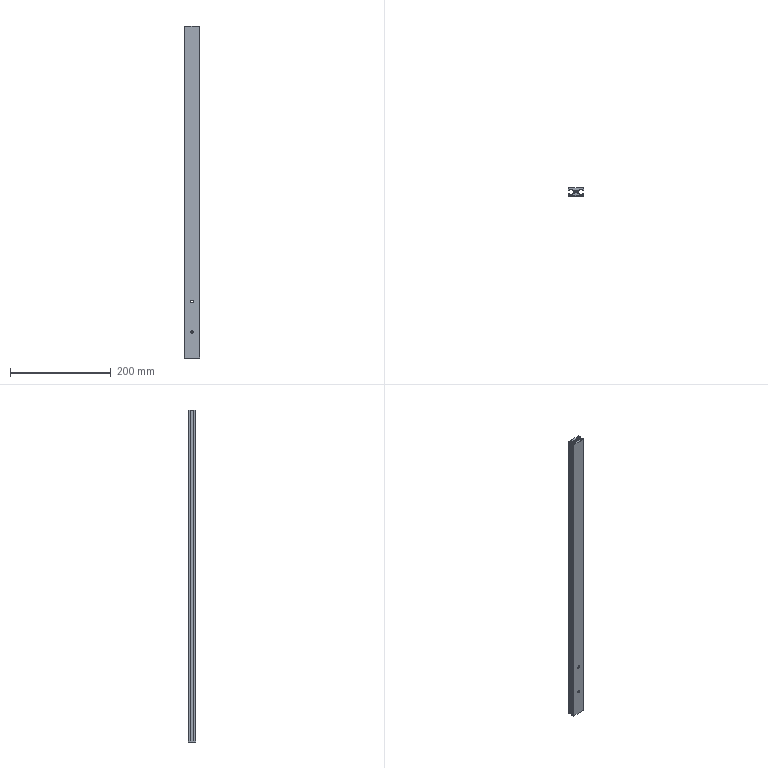Part | SolidWorks | features BaseBody 1, HoleWzd 1, MoveFace 1 | 1 solid | 87 faces | box 30 x 15 x 660 mm | volume 158770 mm3 | plane 46 | cylinder 41 | commonest cylinder face diameters 5 x31 1 x6 2 x4